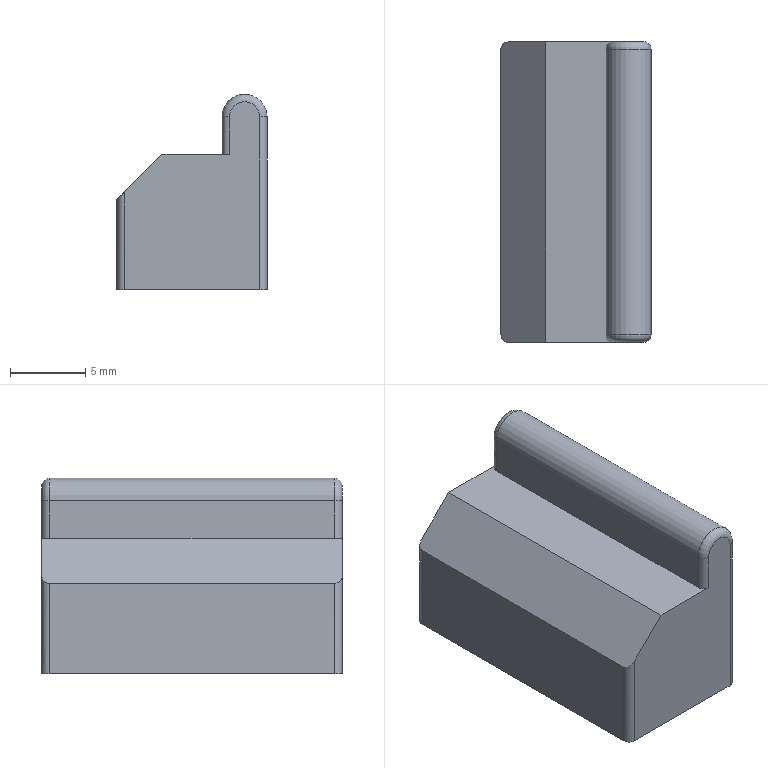NC program | Mastercam | posted with a generic post | part box 10 x 20 x 13 mm
Lines 868 to 2366 of 2366:
(4 BM/BNOS |TOOL - 14|DIA. OFF. - 14|LEN. - 14|TOOL DIA. - 4.)
N1800 T14 M6
N1802 G0 G54 G90 X-9.652 Y.005 C0. B0. S7000 M3
N1804 G43 H14 Z36.433
N1806 Z16.5
N1808 Z6.5
N1810 G1 Z-3.5 F600.
N1812 Y.021 Z-3.157 F3000.
N1814 Y.079 Z-2.784
N1816 Y.144 Z-2.521
N1818 Y.236 Z-2.248
N1820 Y.358 Z-1.968
N1822 Y.513 Z-1.685
N1824 Y.704 Z-1.403
N1826 Y.933 Z-1.128
N1828 Y1.131 Z-.93
N1830 Y1.351 Z-.743
N1832 Y1.593 Z-.571
N1834 Y1.855 Z-.416
N1836 Y2.136 Z-.282
N1838 Y2.434 Z-.171
N1840 Y2.744 Z-.087
N1842 Y3.065 Z-.032
N1844 Y3.391 Z-.006
N1846 Y3.718 Z-.011
N1848 Y4.043 Z-.047
N1850 Y4.36 Z-.112
N1852 Y4.667 Z-.205
N1854 Y4.959 Z-.324
N1856 Y5.235 Z-.465
N1858 Y5.49 Z-.627
N1860 Y5.725 Z-.804
N1862 Y5.938 Z-.995
N1864 Y6.187 Z-1.264
N1866 Y6.396 Z-1.543
N1868 Y6.569 Z-1.827
N1870 Y6.707 Z-2.109
N1872 Y6.813 Z-2.386
N1874 Y6.892 Z-2.654
N1876 Y6.964 Z-3.036
N1878 Y6.994 Z-3.389
N1880 Y6.995 Z-3.5
N1882 X-9.654 Y6.996 Z-3.53
N1884 X-9.66 Z-3.557
N1886 X-9.67 Y6.995 Z-3.579
N1888 X-9.684 Y6.994 Z-3.597
N1890 X-9.702 Y6.993 Z-3.612
N1892 X-9.724 Y6.991 Z-3.622
N1894 X-9.75 Y6.988 Z-3.628
N1896 X-9.781 Y6.985 Z-3.63
N1898 X-9.811 Y6.982 Z-3.628
N1900 X-9.837 Y6.979 Z-3.622
N1902 X-9.859 Y6.976 Z-3.611
N1904 X-9.877 Y6.974 Z-3.597
N1906 X-9.892 Y6.971 Z-3.579
N1908 X-9.902 Y6.97 Z-3.557
N1910 X-9.908 Y6.968 Z-3.53
N1912 X-9.91 Y6.966 Z-3.5
N1914 Y6.949 Z-3.16
N1916 Y6.893 Z-2.79
N1918 Y6.828 Z-2.529
N1920 Y6.736 Z-2.259
N1922 Y6.616 Z-1.981
N1924 Y6.462 Z-1.7
N1926 Y6.273 Z-1.42
N1928 Y6.046 Z-1.148
N1930 Y5.779 Z-.889
N1932 Y5.554 Z-.708
N1934 Y5.307 Z-.542
N1936 Y5.04 Z-.395
N1938 Y4.756 Z-.269
N1940 Y4.456 Z-.168
N1942 Y4.144 Z-.094
N1944 Y3.824 Z-.049
N1946 Y3.5 Z-.034
N1948 Y3.176 Z-.049
N1950 Y2.856 Z-.094
N1952 Y2.544 Z-.168
N1954 Y2.244 Z-.269
N1956 Y1.96 Z-.395
N1958 Y1.693 Z-.542
N1960 Y1.446 Z-.708
N1962 Y1.221 Z-.889
N1964 Y.954 Z-1.148
N1966 Y.727 Z-1.42
N1968 Y.538 Z-1.7
N1970 Y.384 Z-1.981
N1972 Y.264 Z-2.259
N1974 Y.172 Z-2.529
N1976 Y.107 Z-2.79
N1978 Y.051 Z-3.16
N1980 Y.034 Z-3.5
N1982 X-9.912 Y.033 Z-3.531
N1984 X-9.918 Z-3.559
N1986 X-9.928 Y.034 Z-3.582
N1988 X-9.942 Y.036 Z-3.601
N1990 X-9.961 Y.039 Z-3.615
N1992 X-9.983 Y.044 Z-3.626
N1994 X-10.01 Y.05 Z-3.632
N1996 X-10.041 Y.056 Z-3.634
N1998 X-10.072 Y.063 Z-3.632
N2000 X-10.098 Y.069 Z-3.626
N2002 X-10.121 Y.075 Z-3.615
N2004 X-10.139 Y.08 Z-3.601
N2006 X-10.153 Y.084 Z-3.582
N2008 X-10.164 Y.087 Z-3.559
N2010 X-10.17 Y.09 Z-3.531
N2012 X-10.172 Y.092 Z-3.5
N2014 Y.108 Z-3.166
N2016 Y.164 Z-2.802
N2018 Y.228 Z-2.546
N2020 Y.318 Z-2.28
N2022 Y.437 Z-2.007
N2024 Y.588 Z-1.73
N2026 Y.774 Z-1.455
N2028 Y.997 Z-1.187
N2030 Y1.259 Z-.932
N2032 Y1.481 Z-.755
N2034 Y1.724 Z-.592
N2036 Y1.986 Z-.447
N2038 Y2.265 Z-.324
N2040 Y2.56 Z-.224
N2042 Y2.867 Z-.151
N2044 Y3.181 Z-.107
N2046 Y3.5 Z-.092
N2048 Y3.819 Z-.107
N2050 Y4.133 Z-.151
N2052 Y4.44 Z-.224
N2054 Y4.735 Z-.324
N2056 Y5.014 Z-.447
N2058 Y5.276 Z-.592
N2060 Y5.519 Z-.755
N2062 Y5.741 Z-.932
N2064 Y6.003 Z-1.187
N2066 Y6.226 Z-1.455
N2068 Y6.412 Z-1.73
N2070 Y6.563 Z-2.007
N2072 Y6.682 Z-2.28
N2074 Y6.772 Z-2.546
N2076 Y6.836 Z-2.802
N2078 Y6.892 Z-3.166
N2080 Y6.908 Z-3.5
N2082 X-10.174 Y6.909 Z-3.532
N2084 X-10.18 Y6.908 Z-3.56
N2086 X-10.19 Y6.906 Z-3.584
N2088 X-10.205 Y6.902 Z-3.604
N2090 X-10.223 Y6.897 Z-3.619
N2092 X-10.245 Y6.889 Z-3.629
N2094 X-10.272 Y6.881 Z-3.636
N2096 X-10.303 Y6.87 Z-3.638
N2098 X-10.333 Y6.86 Z-3.636
N2100 X-10.36 Y6.851 Z-3.629
N2102 X-10.382 Y6.842 Z-3.619
N2104 X-10.401 Y6.835 Z-3.604
N2106 X-10.415 Y6.83 Z-3.584
N2108 X-10.425 Y6.825 Z-3.56
N2110 X-10.432 Y6.821 Z-3.532
N2112 X-10.434 Y6.819 Z-3.5
N2114 Y6.803 Z-3.174
N2116 Y6.749 Z-2.821
N2118 Y6.686 Z-2.571
N2120 Y6.599 Z-2.311
N2122 Y6.483 Z-2.046
N2124 Y6.337 Z-1.776
N2126 Y6.155 Z-1.509
N2128 Y5.938 Z-1.247
N2130 Y5.682 Z-.999
N2132 Y5.541 Z-.882
N2134 Y5.311 Z-.719
N2136 Y5.062 Z-.571
N2138 Y4.795 Z-.444
N2140 Y4.512 Z-.339
N2142 Y4.217 Z-.259
N2144 Y3.913 Z-.207
N2146 Y3.604 Z-.182
N2148 Y3.293 Z-.187
N2150 Y2.985 Z-.221
N2152 Y2.683 Z-.283
N2154 Y2.392 Z-.371
N2156 Y2.114 Z-.484
N2158 Y1.853 Z-.618
N2160 Y1.61 Z-.771
N2162 Y1.459 Z-.882
N2164 Y1.185 Z-1.121
N2166 Y.949 Z-1.377
N2168 Y.75 Z-1.642
N2170 Y.586 Z-1.911
N2172 Y.455 Z-2.179
N2174 Y.354 Z-2.442
N2176 Y.28 Z-2.697
N2178 Y.21 Z-3.059
N2180 Y.183 Z-3.395
N2182 Y.181 Z-3.5
N2184 X-10.436 Z-3.533
N2186 X-10.442 Y.183 Z-3.562
N2188 X-10.452 Y.187 Z-3.586
N2190 X-10.466 Y.193 Z-3.606
N2192 X-10.484 Y.201 Z-3.621
N2194 X-10.505 Y.211 Z-3.632
N2196 X-10.531 Y.222 Z-3.639
N2198 X-10.561 Y.236 Z-3.641
N2200 X-10.591 Y.25 Z-3.639
N2202 X-10.617 Y.263 Z-3.632
N2204 X-10.639 Y.273 Z-3.621
N2206 X-10.657 Y.282 Z-3.606
N2208 X-10.671 Y.289 Z-3.586
N2210 X-10.681 Y.295 Z-3.562
N2212 X-10.687 Y.299 Z-3.533
N2214 X-10.689 Y.301 Z-3.5
N2216 X-10.69 Y.317 Z-3.186
N2218 Y.369 Z-2.845
N2220 Y.429 Z-2.604
N2222 Y.513 Z-2.355
N2224 Y.625 Z-2.098
N2226 X-10.689 Y.766 Z-1.839
N2228 X-10.69 Y.941 Z-1.581
N2230 Y1.151 Z-1.329
N2232 Y1.397 Z-1.09
N2234 Y1.679 Z-.87
N2236 X-10.689 Y1.833 Z-.77
N2238 Y1.995 Z-.677
N2240 X-10.69 Y2.252 Z-.555
N2242 Y2.524 Z-.454
N2244 Y2.809 Z-.377
N2246 Y3.102 Z-.326
N2248 X-10.689 Y3.4 Z-.303
N2250 X-10.69 Y3.7 Z-.307
N2252 Y3.997 Z-.34
N2254 Y4.287 Z-.4
N2256 Y4.568 Z-.485
N2258 Y4.836 Z-.593
N2260 X-10.689 Y5.005 Z-.677
N2262 Y5.167 Z-.77
N2264 X-10.69 Y5.321 Z-.87
N2266 Y5.603 Z-1.09
N2268 Y5.849 Z-1.329
N2270 Y6.059 Z-1.581
N2272 X-10.689 Y6.234 Z-1.839
N2274 X-10.69 Y6.375 Z-2.098
N2276 Y6.487 Z-2.355
N2278 Y6.571 Z-2.604
N2280 Y6.653 Z-2.962
N2282 Y6.692 Z-3.294
N2284 X-10.689 Y6.699 Z-3.5
N2286 X-10.691 Z-3.534
N2288 X-10.697 Y6.696 Z-3.563
N2290 X-10.707 Y6.692 Z-3.588
N2292 X-10.72 Y6.684 Z-3.608
N2294 X-10.737 Y6.674 Z-3.623
N2296 X-10.758 Y6.662 Z-3.635
N2298 X-10.783 Y6.647 Z-3.641
N2300 X-10.812 Y6.629 Z-3.644
N2302 X-10.84 Y6.612 Z-3.641
N2304 X-10.865 Y6.596 Z-3.635
N2306 X-10.886 Y6.583 Z-3.623
N2308 X-10.903 Y6.571 Z-3.608
N2310 X-10.917 Y6.562 Z-3.587
N2312 X-10.926 Y6.555 Z-3.563
N2314 X-10.932 Y6.551 Z-3.534
N2316 X-10.934 Y6.548 Z-3.5
N2318 Y6.533 Z-3.201
N2320 Y6.483 Z-2.876
N2322 Y6.389 Z-2.529
N2324 Y6.296 Z-2.287
N2326 Y6.176 Z-2.041
N2328 Y6.025 Z-1.794
N2330 Y5.842 Z-1.55
N2332 X-10.935 Y5.625 Z-1.316
N2334 X-10.934 Y5.374 Z-1.097
N2336 Y5.089 Z-.899
N2338 Y4.934 Z-.811
N2340 Y4.772 Z-.731
N2342 Y4.604 Z-.659
N2344 Y4.43 Z-.598
N2346 X-10.935 Y4.25 Z-.546
N2348 X-10.934 Y4.066 Z-.506
N2350 Y3.879 Z-.476
N2352 Y3.69 Z-.458
N2354 Y3.5 Z-.452
N2356 Y3.31 Z-.458
N2358 Y3.121 Z-.476
N2360 Y2.934 Z-.506
N2362 X-10.935 Y2.75 Z-.546
N2364 X-10.934 Y2.57 Z-.598
N2366 Y2.396 Z-.659
N2368 Y2.228 Z-.731
N2370 Y2.066 Z-.811
N2372 Y1.911 Z-.899
N2374 Y1.626 Z-1.097
N2376 X-10.935 Y1.375 Z-1.316
N2378 X-10.934 Y1.158 Z-1.55
N2380 Y.975 Z-1.794
N2382 Y.824 Z-2.041
N2384 Y.704 Z-2.287
N2386 Y.611 Z-2.529
N2388 Y.517 Z-2.876
N2390 Y.467 Z-3.201
N2392 Y.452 Z-3.5
N2394 X-10.936 Z-3.534
N2396 X-10.941 Y.455 Z-3.563
N2398 X-10.95 Y.461 Z-3.588
N2400 X-10.962 Y.47 Z-3.609
N2402 X-10.978 Y.482 Z-3.625
N2404 X-10.998 Y.497 Z-3.636
N2406 X-11.021 Y.515 Z-3.643
N2408 X-11.048 Y.536 Z-3.645
N2410 X-11.074 Y.557 Z-3.643
N2412 X-11.098 Y.576 Z-3.636
N2414 X-11.117 Y.592 Z-3.625
N2416 X-11.133 Y.606 Z-3.609
N2418 X-11.146 Y.616 Z-3.588
N2420 X-11.155 Y.624 Z-3.563
N2422 X-11.16 Y.63 Z-3.534
N2424 X-11.162 Y.632 Z-3.5
N2426 Y.638 Z-3.315
N2428 Y.674 Z-3.017
N2430 Y.747 Z-2.697
N2432 Y.823 Z-2.473
N2434 Y.922 Z-2.243
N2436 Y1.049 Z-2.011
N2438 Y1.206 Z-1.779
N2440 Y1.394 Z-1.554
N2442 Y1.615 Z-1.34
N2444 Y1.867 Z-1.143
N2446 Y2.15 Z-.97
N2448 Y2.303 Z-.894
N2450 Y2.461 Z-.827
N2452 Y2.625 Z-.769
N2454 Y2.794 Z-.721
N2456 Y2.967 Z-.683
N2458 Y3.143 Z-.655
N2460 Y3.321 Z-.638
N2462 Y3.5 Z-.632
N2464 Y3.679 Z-.638
N2466 Y3.857 Z-.655
N2468 Y4.033 Z-.683
N2470 Y4.206 Z-.721
N2472 Y4.375 Z-.769
N2474 Y4.539 Z-.827
N2476 Y4.697 Z-.894
N2478 Y4.85 Z-.97
N2480 Y5.133 Z-1.143
N2482 Y5.385 Z-1.34
N2484 Y5.606 Z-1.554
N2486 Y5.794 Z-1.779
N2488 Y5.951 Z-2.011
N2490 Y6.078 Z-2.243
N2492 Y6.177 Z-2.473
N2494 Y6.282 Z-2.806
N2496 Y6.342 Z-3.119
N2498 Y6.362 Z-3.315
N2500 Y6.368 Z-3.5
N2502 X-11.163 Y6.367 Z-3.534
N2504 X-11.168 Y6.363 Z-3.564
N2506 X-11.176 Y6.356 Z-3.589
N2508 X-11.187 Y6.346 Z-3.609
N2510 X-11.202 Y6.332 Z-3.625
N2512 X-11.22 Y6.314 Z-3.636
N2514 X-11.241 Y6.294 Z-3.643
N2516 X-11.265 Y6.27 Z-3.646
N2518 X-11.289 Y6.245 Z-3.643
N2520 X-11.31 Y6.224 Z-3.636
N2522 X-11.327 Y6.206 Z-3.625
N2524 X-11.342 Y6.191 Z-3.609
N2526 X-11.353 Y6.179 Z-3.589
N2528 X-11.361 Y6.17 Z-3.564
N2530 X-11.366 Y6.164 Z-3.534
N2532 X-11.368 Y6.162 Z-3.5
N2534 Y6.156 Z-3.328
N2536 Y6.138 Z-3.147
N2538 Y6.105 Z-2.955
N2540 Y6.022 Z-2.652
N2542 Y5.892 Z-2.334
N2544 Y5.775 Z-2.118
N2546 Y5.629 Z-1.903
N2548 Y5.454 Z-1.694
N2550 Y5.25 Z-1.495
N2552 Y5.015 Z-1.312
N2554 Y4.753 Z-1.151
N2556 Y4.464 Z-1.019
N2558 Y4.155 Z-.921
N2560 Y3.995 Z-.885
N2562 Y3.831 Z-.859
N2564 Y3.666 Z-.844
N2566 Y3.5 Z-.838
N2568 Y3.334 Z-.844
N2570 Y3.169 Z-.859
N2572 Y3.005 Z-.885
N2574 Y2.688 Z-.966
N2576 Y2.389 Z-1.082
N2578 Y2.113 Z-1.228
N2580 Y1.864 Z-1.401
N2582 Y1.644 Z-1.593
N2584 Y1.454 Z-1.798
N2586 Y1.294 Z-2.01
N2588 Y1.163 Z-2.226
N2590 Y1.058 Z-2.441
N2592 Y.945 Z-2.755
N2594 Y.895 Z-2.955
N2596 Y.862 Z-3.147
N2598 Y.844 Z-3.328
N2600 Y.838 Z-3.5
N2602 X-11.369 Y.839 Z-3.534
N2604 X-11.373 Y.843 Z-3.563
N2606 X-11.38 Y.851 Z-3.588
N2608 X-11.39 Y.863 Z-3.609
N2610 X-11.403 Y.879 Z-3.625
N2612 X-11.418 Y.898 Z-3.636
N2614 X-11.437 Y.921 Z-3.643
N2616 X-11.458 Y.947 Z-3.645
N2618 X-11.479 Y.974 Z-3.643
N2620 X-11.497 Y.997 Z-3.636
N2622 X-11.513 Y1.017 Z-3.625
N2624 X-11.525 Y1.034 Z-3.609
N2626 X-11.535 Y1.047 Z-3.588
N2628 X-11.542 Y1.057 Z-3.563
N2630 X-11.546 Y1.063 Z-3.534
N2632 X-11.548 Y1.066 Z-3.5
N2634 Y1.071 Z-3.343
N2636 Y1.088 Z-3.177
N2638 Y1.118 Z-3.002
N2640 Y1.164 Z-2.819
N2642 Y1.228 Z-2.629
N2644 Y1.363 Z-2.335
N2646 Y1.483 Z-2.138
N2648 Y1.63 Z-1.943
N2650 Y1.803 Z-1.756
N2652 Y2.004 Z-1.581
N2654 Y2.231 Z-1.423
N2656 Y2.484 Z-1.289
N2658 Y2.758 Z-1.183
N2660 Y3.048 Z-1.109
N2662 Y3.348 Z-1.071
N2664 Y3.652
N2666 Y3.952 Z-1.109
N2668 Y4.242 Z-1.183
N2670 Y4.516 Z-1.289
N2672 Y4.769 Z-1.423
N2674 Y4.996 Z-1.581
N2676 Y5.197 Z-1.756
N2678 Y5.37 Z-1.943
N2680 Y5.517 Z-2.138
N2682 Y5.637 Z-2.335
N2684 Y5.772 Z-2.629
N2686 Y5.836 Z-2.819
N2688 Y5.882 Z-3.002
N2690 Y5.912 Z-3.177
N2692 Y5.929 Z-3.343
N2694 Y5.934 Z-3.5
N2696 X-11.549 Y5.933 Z-3.534
N2698 X-11.553 Y5.929 Z-3.563
N2700 X-11.558 Y5.92 Z-3.587
N2702 X-11.567 Y5.908 Z-3.608
N2704 X-11.577 Y5.892 Z-3.623
N2706 X-11.59 Y5.872 Z-3.635
N2708 X-11.606 Y5.847 Z-3.641
N2710 X-11.623 Y5.819 Z-3.644
N2712 X-11.641 Y5.79 Z-3.641
N2714 X-11.656 Y5.765 Z-3.635
N2716 X-11.669 Y5.744 Z-3.623
N2718 X-11.68 Y5.726 Z-3.608
N2720 X-11.688 Y5.712 Z-3.587
N2722 X-11.694 Y5.701 Z-3.563
N2724 X-11.698 Y5.694 Z-3.534
N2726 X-11.699 Y5.689 Z-3.5
N2728 Y5.67 Z-3.209
N2730 Y5.642 Z-3.052
N2732 Y5.601 Z-2.887
N2734 Y5.544 Z-2.716
N2736 Y5.468 Z-2.541
N2738 Y5.371 Z-2.363
N2740 Y5.251 Z-2.187
N2742 Y5.107 Z-2.015
N2744 Y4.939 Z-1.851
N2746 Y4.747 Z-1.7
N2748 Y4.53 Z-1.568
N2750 Y4.293 Z-1.46
N2752 Y4.039 Z-1.379
N2754 Y3.773 Z-1.328
N2756 Y3.5 Z-1.311
N2758 Y3.227 Z-1.328
N2760 Y2.961 Z-1.379
N2762 Y2.707 Z-1.46
N2764 Y2.47 Z-1.568
N2766 Y2.253 Z-1.7
N2768 Y2.154 Z-1.774
N2770 Y1.974 Z-1.931
N2772 Y1.818 Z-2.1
N2774 Y1.686 Z-2.274
N2776 Y1.532 Z-2.541
N2778 Y1.456 Z-2.716
N2780 Y1.399 Z-2.887
N2782 Y1.358 Z-3.052
N2784 Y1.33 Z-3.209
N2786 Y1.311 Z-3.5
N2788 X-11.7 Y1.31 Z-3.533
N2790 X-11.703 Y1.314 Z-3.562
N2792 X-11.707 Y1.323 Z-3.586
N2794 X-11.714 Y1.335 Z-3.606
N2796 X-11.722 Y1.352 Z-3.621
N2798 X-11.733 Y1.373 Z-3.632
N2800 X-11.745 Y1.399 Z-3.639
N2802 X-11.759 Y1.429 Z-3.641
N2804 X-11.773 Y1.459 Z-3.639
N2806 X-11.785 Y1.485 Z-3.632
N2808 X-11.796 Y1.508 Z-3.621
N2810 X-11.804 Y1.527 Z-3.606
N2812 X-11.811 Y1.543 Z-3.586
N2814 X-11.815 Y1.554 Z-3.562
N2816 X-11.818 Y1.562 Z-3.533
N2818 X-11.819 Y1.566 Z-3.5
N2820 Y1.584 Z-3.243
N2822 Y1.608 Z-3.104
N2824 X-11.82 Y1.645 Z-2.959
N2826 X-11.819 Y1.695 Z-2.808
N2828 Y1.802 Z-2.574
N2830 Y1.898 Z-2.418
N2832 Y2.014 Z-2.264
N2834 X-11.82 Y2.152 Z-2.115
N2836 X-11.819 Y2.311 Z-1.976
N2838 Y2.492 Z-1.85
N2840 Y2.693 Z-1.743
N2842 Y2.91 Z-1.659
N2844 Y3.141 Z-1.601
N2846 Y3.379 Z-1.57
N2848 Y3.621
N2850 Y3.859 Z-1.601
N2852 Y4.09 Z-1.659
N2854 Y4.307 Z-1.743
N2856 Y4.508 Z-1.85
N2858 Y4.689 Z-1.976
N2860 X-11.82 Y4.848 Z-2.115
N2862 X-11.819 Y4.986 Z-2.264
N2864 Y5.102 Z-2.418
N2866 Y5.198 Z-2.574
N2868 Y5.305 Z-2.808
N2870 X-11.82 Y5.355 Z-2.959
N2872 X-11.819 Y5.392 Z-3.104
N2874 Y5.416 Z-3.243
N2876 Y5.434 Z-3.5
N2878 X-11.82 Z-3.532
N2880 X-11.822 Y5.43 Z-3.56
N2882 X-11.825 Y5.421 Z-3.584
N2884 X-11.83 Y5.408 Z-3.603
N2886 X-11.836 Y5.391 Z-3.618
N2888 X-11.844 Y5.369 Z-3.629
N2890 X-11.853 Y5.343 Z-3.636
N2892 X-11.863 Y5.312 Z-3.638
N2894 X-11.874 Y5.281 Z-3.636
N2896 X-11.883 Y5.254 Z-3.629
N2898 X-11.891 Y5.231 Z-3.618
N2900 X-11.897 Y5.212 Z-3.603
N2902 X-11.902 Y5.196 Z-3.584
N2904 X-11.905 Y5.184 Z-3.56
N2906 X-11.907 Y5.176 Z-3.532
N2908 X-11.908 Y5.172 Z-3.5
N2910 Y5.157 Z-3.278
N2912 Y5.104 Z-3.032
N2914 Y5.06 Z-2.902
N2916 Y4.968 Z-2.7
N2918 Y4.837 Z-2.497
N2920 Y4.665 Z-2.302
N2922 Y4.528 Z-2.182
N2924 Y4.371 Z-2.073
N2926 Y4.198 Z-1.981
N2928 Y4.01 Z-1.909
N2930 Y3.811 Z-1.858
N2932 Y3.604 Z-1.832
N2934 Y3.396
N2936 Y3.189 Z-1.858
N2938 Y2.99 Z-1.909
N2940 Y2.802 Z-1.981
N2942 Y2.629 Z-2.073
N2944 Y2.472 Z-2.182
N2946 Y2.273 Z-2.366
N2948 Y2.115 Z-2.564
N2950 Y1.997 Z-2.767
N2952 Y1.94 Z-2.902
N2954 Y1.896 Z-3.032
N2956 Y1.843 Z-3.278
N2958 Y1.828 Z-3.5
N2960 Z-3.531
N2962 X-11.91 Y1.832 Z-3.559
N2964 X-11.912 Y1.841 Z-3.582
N2966 X-11.915 Y1.854 Z-3.6
N2968 X-11.919 Y1.871 Z-3.615
N2970 X-11.924 Y1.893 Z-3.626
N2972 X-11.93 Y1.919 Z-3.632
N2974 X-11.937 Y1.95 Z-3.634
N2976 X-11.944 Y1.981 Z-3.632
N2978 X-11.95 Y2.008 Z-3.626
N2980 X-11.955 Y2.031 Z-3.615
N2982 X-11.959 Y2.051 Z-3.6
N2984 X-11.962 Y2.066 Z-3.582
N2986 X-11.964 Y2.078 Z-3.559
N2988 X-11.966 Y2.086 Z-3.531
N2990 Y2.09 Z-3.5
N2992 Y2.103 Z-3.313
N2994 Y2.148 Z-3.106
N2996 Y2.233 Z-2.882
N2998 Y2.295 Z-2.768
N3000 Y2.417 Z-2.599
N3002 Y2.574 Z-2.439
N3004 Y2.765 Z-2.297
N3006 Y2.912 Z-2.219
N3008 Y3.07 Z-2.158
N3010 Y3.238 Z-2.116
N3012 Y3.412 Z-2.093
N3014 Y3.588
N3016 Y3.762 Z-2.116
N3018 Y3.93 Z-2.158
N3020 Y4.088 Z-2.219
N3022 Y4.235 Z-2.297
N3024 Y4.426 Z-2.439
N3026 Y4.583 Z-2.599
N3028 Y4.705 Z-2.768
N3030 Y4.767 Z-2.882
N3032 Y4.852 Z-3.106
N3034 Y4.897 Z-3.313
N3036 Y4.91 Z-3.5
N3038 Z-3.53
N3040 X-11.967 Y4.906 Z-3.557
N3042 X-11.968 Y4.897 Z-3.579
N3044 X-11.97 Y4.884 Z-3.597
N3046 X-11.972 Y4.867 Z-3.611
N3048 X-11.974 Y4.846 Z-3.621
N3050 X-11.977 Y4.82 Z-3.627
N3052 X-11.981 Y4.79 Z-3.629
N3054 X-11.984 Y4.759 Z-3.627
N3056 X-11.987 Y4.733 Z-3.621
N3058 X-11.99 Y4.71 Z-3.611
N3060 X-11.992 Y4.691 Z-3.597
N3062 X-11.993 Y4.675 Z-3.579
N3064 X-11.994 Y4.664 Z-3.557
N3066 X-11.995 Y4.656 Z-3.53
N3068 Y4.652 Z-3.5
N3070 Y4.641 Z-3.347
N3072 Y4.605 Z-3.178
N3074 Y4.535 Z-2.995
N3076 Y4.484 Z-2.902
N3078 Y4.385 Z-2.764
N3080 Y4.257 Z-2.633
N3082 Y4.1 Z-2.517
N3084 Y3.917 Z-2.427
N3086 Y3.714 Z-2.369
N3088 Y3.5 Z-2.348
N3090 Y3.286 Z-2.369
N3092 Y3.083 Z-2.427
N3094 Y2.9 Z-2.517
N3096 Y2.743 Z-2.633
N3098 Y2.615 Z-2.764
N3100 Y2.516 Z-2.902
N3102 Y2.425 Z-3.088
N3104 Y2.374 Z-3.264
N3106 Y2.351 Z-3.426
N3108 Y2.348 Z-3.5
N3110 G0 Z6.5
N3112 Z16.5
N3114 Z36.433
N3116 X9.652 Y6.995
N3118 Z16.5
N3120 Z6.5
N3122 G1 Z-3.5 F600.
N3124 Y6.979 Z-3.157 F3000.
N3126 Y6.921 Z-2.784
N3128 Y6.856 Z-2.521
N3130 Y6.764 Z-2.248
N3132 Y6.642 Z-1.968
N3134 Y6.487 Z-1.685
N3136 Y6.296 Z-1.403
N3138 Y6.067 Z-1.128
N3140 Y5.869 Z-.93
N3142 Y5.649 Z-.743
N3144 Y5.407 Z-.571
N3146 Y5.145 Z-.416
N3148 Y4.864 Z-.282
N3150 Y4.566 Z-.171
N3152 Y4.256 Z-.087
N3154 Y3.935 Z-.032
N3156 Y3.609 Z-.006
N3158 Y3.282 Z-.011
N3160 Y2.957 Z-.047
N3162 Y2.64 Z-.112
N3164 Y2.333 Z-.205
N3166 Y2.041 Z-.324
N3168 Y1.765 Z-.465
N3170 Y1.51 Z-.627
N3172 Y1.275 Z-.804
N3174 Y1.062 Z-.995
N3176 Y.813 Z-1.264
N3178 Y.604 Z-1.543
N3180 Y.431 Z-1.827
N3182 Y.293 Z-2.109
N3184 Y.187 Z-2.386
N3186 Y.108 Z-2.654
N3188 Y.036 Z-3.036
N3190 Y.006 Z-3.389
N3192 Y.005 Z-3.5
N3194 X9.654 Y.004 Z-3.53
N3196 X9.66 Z-3.557
N3198 X9.67 Y.005 Z-3.579
N3200 X9.684 Y.006 Z-3.597
N3202 X9.702 Y.007 Z-3.612
N3204 X9.724 Y.009 Z-3.622
N3206 X9.75 Y.012 Z-3.628
N3208 X9.781 Y.015 Z-3.63
N3210 X9.811 Y.018 Z-3.628
N3212 X9.837 Y.021 Z-3.622
N3214 X9.859 Y.024 Z-3.611
N3216 X9.877 Y.026 Z-3.597
N3218 X9.892 Y.029 Z-3.579
N3220 X9.902 Y.03 Z-3.557
N3222 X9.908 Y.032 Z-3.53
N3224 X9.91 Y.034 Z-3.5
N3226 Y.051 Z-3.16
N3228 Y.107 Z-2.79
N3230 Y.172 Z-2.529
N3232 Y.264 Z-2.259
N3234 Y.384 Z-1.981
N3236 Y.538 Z-1.7
N3238 Y.727 Z-1.42
N3240 Y.954 Z-1.148
N3242 Y1.221 Z-.889
N3244 Y1.446 Z-.708
N3246 Y1.693 Z-.542
N3248 Y1.96 Z-.395
N3250 Y2.244 Z-.269
N3252 Y2.544 Z-.168
N3254 Y2.856 Z-.094
N3256 Y3.176 Z-.049
N3258 Y3.5 Z-.034
N3260 Y3.824 Z-.049
N3262 Y4.144 Z-.094
N3264 Y4.456 Z-.168
N3266 Y4.756 Z-.269
N3268 Y5.04 Z-.395
N3270 Y5.307 Z-.542
N3272 Y5.554 Z-.708
N3274 Y5.779 Z-.889
N3276 Y6.046 Z-1.148
N3278 Y6.273 Z-1.42
N3280 Y6.462 Z-1.7
N3282 Y6.616 Z-1.981
N3284 Y6.736 Z-2.259
N3286 Y6.828 Z-2.529
N3288 Y6.893 Z-2.79
N3290 Y6.949 Z-3.16
N3292 Y6.966 Z-3.5
N3294 X9.912 Y6.967 Z-3.531
N3296 X9.918 Z-3.559
N3298 X9.928 Y6.966 Z-3.582
N3300 X9.942 Y6.964 Z-3.601
N3302 X9.961 Y6.961 Z-3.615
N3304 X9.983 Y6.956 Z-3.626
N3306 X10.01 Y6.95 Z-3.632
N3308 X10.041 Y6.944 Z-3.634
N3310 X10.072 Y6.937 Z-3.632
N3312 X10.098 Y6.931 Z-3.626
N3314 X10.121 Y6.925 Z-3.615
N3316 X10.139 Y6.92 Z-3.601
N3318 X10.153 Y6.916 Z-3.582
N3320 X10.164 Y6.913 Z-3.559
N3322 X10.17 Y6.91 Z-3.531
N3324 X10.172 Y6.908 Z-3.5
N3326 Y6.892 Z-3.166
N3328 Y6.836 Z-2.802
N3330 Y6.772 Z-2.546
N3332 Y6.682 Z-2.28
N3334 Y6.563 Z-2.007
N3336 Y6.412 Z-1.73
N3338 Y6.226 Z-1.455
N3340 Y6.003 Z-1.187
N3342 Y5.741 Z-.932
N3344 Y5.519 Z-.755
N3346 Y5.276 Z-.592
N3348 Y5.014 Z-.447
N3350 Y4.735 Z-.324
N3352 Y4.44 Z-.224
N3354 Y4.133 Z-.151
N3356 Y3.819 Z-.107
N3358 Y3.5 Z-.092
N3360 Y3.181 Z-.107
N3362 Y2.867 Z-.151
N3364 Y2.56 Z-.224
N3366 Y2.265 Z-.324
N3368 Y1.986 Z-.447
N3370 Y1.724 Z-.592
N3372 Y1.481 Z-.755
N3374 Y1.259 Z-.932
N3376 Y.997 Z-1.187
N3378 Y.774 Z-1.455
N3380 Y.588 Z-1.73
N3382 Y.437 Z-2.007
N3384 Y.318 Z-2.28
N3386 Y.228 Z-2.546
N3388 Y.164 Z-2.802
N3390 Y.108 Z-3.166
N3392 Y.092 Z-3.5
N3394 X10.174 Y.091 Z-3.532
N3396 X10.18 Y.092 Z-3.56
N3398 X10.19 Y.094 Z-3.584
N3400 X10.205 Y.098 Z-3.604
N3402 X10.223 Y.103 Z-3.619
N3404 X10.245 Y.111 Z-3.629
N3406 X10.272 Y.119 Z-3.636
N3408 X10.303 Y.13 Z-3.638
N3410 X10.333 Y.14 Z-3.636
N3412 X10.36 Y.149 Z-3.629
N3414 X10.382 Y.158 Z-3.619
N3416 X10.401 Y.165 Z-3.604
N3418 X10.415 Y.17 Z-3.584
N3420 X10.425 Y.175 Z-3.56
N3422 X10.432 Y.179 Z-3.532
N3424 X10.434 Y.181 Z-3.5
N3426 Y.197 Z-3.174
N3428 Y.251 Z-2.821
N3430 Y.314 Z-2.571
N3432 Y.401 Z-2.311
N3434 Y.517 Z-2.046
N3436 Y.663 Z-1.776
N3438 Y.845 Z-1.509
N3440 Y1.062 Z-1.247
N3442 Y1.318 Z-.999
N3444 Y1.459 Z-.882
N3446 Y1.689 Z-.719
N3448 Y1.938 Z-.571
N3450 Y2.205 Z-.444
N3452 Y2.488 Z-.339
N3454 Y2.783 Z-.259
N3456 Y3.087 Z-.207
N3458 Y3.396 Z-.182
N3460 Y3.707 Z-.187
N3462 Y4.015 Z-.221
N3464 Y4.317 Z-.283
N3466 Y4.608 Z-.371
N3468 Y4.886 Z-.484
N3470 Y5.147 Z-.618
N3472 Y5.39 Z-.771
N3474 Y5.541 Z-.882
N3476 Y5.815 Z-1.121
N3478 Y6.051 Z-1.377
N3480 Y6.25 Z-1.642
N3482 Y6.414 Z-1.911
N3484 Y6.545 Z-2.179
N3486 Y6.646 Z-2.442
N3488 Y6.72 Z-2.697
N3490 Y6.79 Z-3.059
N3492 Y6.817 Z-3.395
N3494 Y6.819 Z-3.5
N3496 X10.436 Z-3.533
N3498 X10.442 Y6.817 Z-3.562
N3500 X10.452 Y6.813 Z-3.586
N3502 X10.466 Y6.807 Z-3.606
N3504 X10.484 Y6.799 Z-3.621
N3506 X10.505 Y6.789 Z-3.632
N3508 X10.531 Y6.778 Z-3.639
N3510 X10.561 Y6.764 Z-3.641
N3512 X10.591 Y6.75 Z-3.639
N3514 X10.617 Y6.737 Z-3.632
N3516 X10.639 Y6.727 Z-3.621
N3518 X10.657 Y6.718 Z-3.606
N3520 X10.671 Y6.711 Z-3.586
N3522 X10.681 Y6.705 Z-3.562
N3524 X10.687 Y6.701 Z-3.533
N3526 X10.689 Y6.699 Z-3.5
N3528 X10.69 Y6.683 Z-3.186
N3530 Y6.631 Z-2.845
N3532 Y6.571 Z-2.604
N3534 Y6.487 Z-2.355
N3536 Y6.375 Z-2.098
N3538 X10.689 Y6.234 Z-1.839
N3540 X10.69 Y6.059 Z-1.581
N3542 Y5.849 Z-1.329
N3544 Y5.603 Z-1.09
N3546 Y5.321 Z-.87
N3548 X10.689 Y5.167 Z-.77
N3550 Y5.005 Z-.677
N3552 X10.69 Y4.748 Z-.555
N3554 Y4.476 Z-.454
N3556 Y4.191 Z-.377
N3558 Y3.898 Z-.326
N3560 X10.689 Y3.6 Z-.303
N3562 X10.69 Y3.3 Z-.307
N3564 Y3.003 Z-.34
N3566 Y2.713 Z-.4
N3568 Y2.432 Z-.485
N3570 Y2.164 Z-.593
N3572 X10.689 Y1.995 Z-.677
N3574 Y1.833 Z-.77
N3576 X10.69 Y1.679 Z-.87
N3578 Y1.397 Z-1.09
N3580 Y1.151 Z-1.329
N3582 Y.941 Z-1.581
N3584 X10.689 Y.766 Z-1.839
N3586 X10.69 Y.625 Z-2.098
N3588 Y.513 Z-2.355
N3590 Y.429 Z-2.604
N3592 Y.347 Z-2.962
N3594 Y.308 Z-3.294
N3596 X10.689 Y.301 Z-3.5
N3598 X10.691 Z-3.534
N3600 X10.697 Y.304 Z-3.563
N3602 X10.707 Y.308 Z-3.588
N3604 X10.72 Y.316 Z-3.608
N3606 X10.737 Y.326 Z-3.623
N3608 X10.758 Y.338 Z-3.635
N3610 X10.783 Y.353 Z-3.641
N3612 X10.812 Y.371 Z-3.644
N3614 X10.84 Y.388 Z-3.641
N3616 X10.865 Y.404 Z-3.635
N3618 X10.886 Y.417 Z-3.623
N3620 X10.903 Y.429 Z-3.608
N3622 X10.917 Y.438 Z-3.587
N3624 X10.926 Y.445 Z-3.563
N3626 X10.932 Y.449 Z-3.534
N3628 X10.934 Y.452 Z-3.5
N3630 Y.467 Z-3.201
N3632 Y.517 Z-2.876
N3634 Y.611 Z-2.529
N3636 Y.704 Z-2.287
N3638 Y.824 Z-2.041
N3640 Y.975 Z-1.794
N3642 Y1.158 Z-1.55
N3644 X10.935 Y1.375 Z-1.316
N3646 X10.934 Y1.626 Z-1.097
N3648 Y1.911 Z-.899
N3650 Y2.066 Z-.811
N3652 Y2.228 Z-.731
N3654 Y2.396 Z-.659
N3656 Y2.57 Z-.598
N3658 X10.935 Y2.75 Z-.546
N3660 X10.934 Y2.934 Z-.506
N3662 Y3.121 Z-.476
N3664 Y3.31 Z-.458
N3666 Y3.5 Z-.452
N3668 Y3.69 Z-.458
N3670 Y3.879 Z-.476
N3672 Y4.066 Z-.506
N3674 X10.935 Y4.25 Z-.546
N3676 X10.934 Y4.43 Z-.598
N3678 Y4.604 Z-.659
N3680 Y4.772 Z-.731
N3682 Y4.934 Z-.811
N3684 Y5.089 Z-.899
N3686 Y5.374 Z-1.097
N3688 X10.935 Y5.625 Z-1.316
N3690 X10.934 Y5.842 Z-1.55
N3692 Y6.025 Z-1.794
N3694 Y6.176 Z-2.041
N3696 Y6.296 Z-2.287
N3698 Y6.389 Z-2.529
N3700 Y6.483 Z-2.876
N3702 Y6.533 Z-3.201
N3704 Y6.548 Z-3.5
N3706 X10.936 Z-3.534
N3708 X10.941 Y6.545 Z-3.563
N3710 X10.95 Y6.539 Z-3.588
N3712 X10.962 Y6.53 Z-3.609
N3714 X10.978 Y6.518 Z-3.625
N3716 X10.998 Y6.503 Z-3.636
N3718 X11.021 Y6.485 Z-3.643
N3720 X11.048 Y6.464 Z-3.645
N3722 X11.074 Y6.443 Z-3.643
N3724 X11.098 Y6.424 Z-3.636
N3726 X11.117 Y6.408 Z-3.625
N3728 X11.133 Y6.394 Z-3.609
N3730 X11.146 Y6.384 Z-3.588
N3732 X11.155 Y6.376 Z-3.563
N3734 X11.16 Y6.37 Z-3.534
N3736 X11.162 Y6.368 Z-3.5
N3738 Y6.362 Z-3.315
N3740 Y6.326 Z-3.017
N3742 Y6.253 Z-2.697
N3744 Y6.177 Z-2.473
N3746 Y6.078 Z-2.243
N3748 Y5.951 Z-2.011
N3750 Y5.794 Z-1.779
N3752 Y5.606 Z-1.554
N3754 Y5.385 Z-1.34
N3756 Y5.133 Z-1.143
N3758 Y4.85 Z-.97
N3760 Y4.697 Z-.894
N3762 Y4.539 Z-.827
N3764 Y4.375 Z-.769
N3766 Y4.206 Z-.721
N3768 Y4.033 Z-.683
N3770 Y3.857 Z-.655
N3772 Y3.679 Z-.638
N3774 Y3.5 Z-.632
N3776 Y3.321 Z-.638
N3778 Y3.143 Z-.655
N3780 Y2.967 Z-.683
N3782 Y2.794 Z-.721
N3784 Y2.625 Z-.769
N3786 Y2.461 Z-.827
N3788 Y2.303 Z-.894
N3790 Y2.15 Z-.97
N3792 Y1.867 Z-1.143
N3794 Y1.615 Z-1.34
N3796 Y1.394 Z-1.554
N3798 Y1.206 Z-1.779
N3800 Y1.049 Z-2.011
N3802 Y.922 Z-2.243
N3804 Y.823 Z-2.473
N3806 Y.718 Z-2.806
N3808 Y.658 Z-3.119
N3810 Y.638 Z-3.315
N3812 Y.632 Z-3.5
N3814 X11.163 Y.633 Z-3.534
N3816 X11.168 Y.637 Z-3.564
N3818 X11.176 Y.644 Z-3.589
N3820 X11.187 Y.654 Z-3.609
N3822 X11.202 Y.668 Z-3.625
N3824 X11.22 Y.686 Z-3.636
N3826 X11.241 Y.706 Z-3.643
N3828 X11.265 Y.73 Z-3.646
N3830 X11.289 Y.755 Z-3.643
N3832 X11.31 Y.776 Z-3.636
N3834 X11.327 Y.794 Z-3.625
N3836 X11.342 Y.809 Z-3.609
N3838 X11.353 Y.821 Z-3.589
N3840 X11.361 Y.83 Z-3.564
N3842 X11.366 Y.836 Z-3.534
N3844 X11.368 Y.838 Z-3.5
N3846 Y.844 Z-3.328
N3848 Y.862 Z-3.147
N3850 Y.895 Z-2.955
N3852 Y.978 Z-2.652
N3854 Y1.108 Z-2.334
N3856 Y1.225 Z-2.118
N3858 Y1.371 Z-1.903
N3860 Y1.546 Z-1.694
N3862 Y1.75 Z-1.495
N3864 Y1.985 Z-1.312
N3866 Y2.247 Z-1.151
N3868 Y2.536 Z-1.019
N3870 Y2.845 Z-.921
N3872 Y3.005 Z-.885
N3874 Y3.169 Z-.859
N3876 Y3.334 Z-.844
N3878 Y3.5 Z-.838
N3880 Y3.666 Z-.844
N3882 Y3.831 Z-.859
N3884 Y3.995 Z-.885
N3886 Y4.312 Z-.966
N3888 Y4.611 Z-1.082
N3890 Y4.887 Z-1.228
N3892 Y5.136 Z-1.401
N3894 Y5.356 Z-1.593
N3896 Y5.546 Z-1.798
N3898 Y5.706 Z-2.01
N3900 Y5.837 Z-2.226
N3902 Y5.942 Z-2.441
N3904 Y6.055 Z-2.755
N3906 Y6.105 Z-2.955
N3908 Y6.138 Z-3.147
N3910 Y6.156 Z-3.328
N3912 Y6.162 Z-3.5
N3914 X11.369 Y6.161 Z-3.534
N3916 X11.373 Y6.157 Z-3.563
N3918 X11.38 Y6.149 Z-3.588
N3920 X11.39 Y6.137 Z-3.609
N3922 X11.403 Y6.121 Z-3.625
N3924 X11.418 Y6.102 Z-3.636
N3926 X11.437 Y6.079 Z-3.643
N3928 X11.458 Y6.053 Z-3.645
N3930 X11.479 Y6.026 Z-3.643
N3932 X11.497 Y6.003 Z-3.636
N3934 X11.513 Y5.983 Z-3.625
N3936 X11.525 Y5.966 Z-3.609
N3938 X11.535 Y5.953 Z-3.588
N3940 X11.542 Y5.943 Z-3.563
N3942 X11.546 Y5.937 Z-3.534
N3944 X11.548 Y5.934 Z-3.5
N3946 Y5.929 Z-3.343
N3948 Y5.912 Z-3.177
N3950 Y5.882 Z-3.002
N3952 Y5.836 Z-2.819
N3954 Y5.772 Z-2.629
N3956 Y5.637 Z-2.335
N3958 Y5.517 Z-2.138
N3960 Y5.37 Z-1.943
N3962 Y5.197 Z-1.756
N3964 Y4.996 Z-1.581
N3966 Y4.769 Z-1.423
N3968 Y4.516 Z-1.289
N3970 Y4.242 Z-1.183
N3972 Y3.952 Z-1.109
N3974 Y3.652 Z-1.071
N3976 Y3.348
N3978 Y3.048 Z-1.109
N3980 Y2.758 Z-1.183
N3982 Y2.484 Z-1.289
N3984 Y2.231 Z-1.423
N3986 Y2.004 Z-1.581
N3988 Y1.803 Z-1.756
N3990 Y1.63 Z-1.943
N3992 Y1.483 Z-2.138
N3994 Y1.363 Z-2.335
N3996 Y1.228 Z-2.629
N3998 Y1.164 Z-2.819
N4000 Y1.118 Z-3.002
N4002 Y1.088 Z-3.177
N4004 Y1.071 Z-3.343
N4006 Y1.066 Z-3.5
N4008 X11.549 Y1.067 Z-3.534
N4010 X11.553 Y1.071 Z-3.563
N4012 X11.558 Y1.08 Z-3.587
N4014 X11.567 Y1.092 Z-3.608
N4016 X11.577 Y1.108 Z-3.623
N4018 X11.59 Y1.128 Z-3.635
N4020 X11.606 Y1.153 Z-3.641
N4022 X11.623 Y1.181 Z-3.644
N4024 X11.641 Y1.21 Z-3.641
N4026 X11.656 Y1.235 Z-3.635
N4028 X11.669 Y1.256 Z-3.623
N4030 X11.68 Y1.274 Z-3.608
N4032 X11.688 Y1.288 Z-3.587
N4034 X11.694 Y1.299 Z-3.563
N4036 X11.698 Y1.306 Z-3.534
N4038 X11.699 Y1.311 Z-3.5
N4040 Y1.33 Z-3.209
N4042 Y1.358 Z-3.052
N4044 Y1.399 Z-2.887
N4046 Y1.456 Z-2.716
N4048 Y1.578 Z-2.452
N4050 Y1.686 Z-2.274
N4052 Y1.818 Z-2.1
N4054 Y1.974 Z-1.931
N4056 Y2.154 Z-1.774
N4058 Y2.359 Z-1.632
N4060 Y2.586 Z-1.511
N4062 Y2.832 Z-1.416
N4064 Y3.093 Z-1.349
N4066 Y3.363 Z-1.315
N4068 Y3.637
N4070 Y3.907 Z-1.349
N4072 Y4.168 Z-1.416
N4074 Y4.414 Z-1.511
N4076 Y4.641 Z-1.632
N4078 Y4.846 Z-1.774
N4080 Y4.939 Z-1.851
N4082 Y5.107 Z-2.015
N4084 Y5.251 Z-2.187
N4086 Y5.371 Z-2.363
N4088 Y5.468 Z-2.541
N4090 Y5.544 Z-2.716
N4092 Y5.601 Z-2.887
N4094 Y5.642 Z-3.052
N4096 Y5.67 Z-3.209
N4098 Y5.689 Z-3.5
N4100 X11.7 Y5.69 Z-3.533
N4102 X11.703 Y5.686 Z-3.562
N4104 X11.707 Y5.677 Z-3.586
N4106 X11.714 Y5.665 Z-3.606
N4108 X11.722 Y5.648 Z-3.621
N4110 X11.733 Y5.627 Z-3.632
N4112 X11.745 Y5.601 Z-3.639
N4114 X11.759 Y5.571 Z-3.641
N4116 X11.773 Y5.541 Z-3.639
N4118 X11.785 Y5.515 Z-3.632
N4120 X11.796 Y5.492 Z-3.621
N4122 X11.804 Y5.473 Z-3.606
N4124 X11.811 Y5.457 Z-3.586
N4126 X11.815 Y5.446 Z-3.562
N4128 X11.818 Y5.438 Z-3.533
N4130 X11.819 Y5.434 Z-3.5
N4132 Y5.416 Z-3.243
N4134 Y5.392 Z-3.104
N4136 X11.82 Y5.355 Z-2.959
N4138 X11.819 Y5.305 Z-2.808
N4140 Y5.198 Z-2.574
N4142 Y5.102 Z-2.418
N4144 Y4.986 Z-2.264
N4146 X11.82 Y4.848 Z-2.115
N4148 X11.819 Y4.689 Z-1.976
N4150 Y4.508 Z-1.85
N4152 Y4.307 Z-1.743
N4154 Y4.09 Z-1.659
N4156 Y3.859 Z-1.601
N4158 Y3.621 Z-1.57
N4160 Y3.379
N4162 Y3.141 Z-1.601
N4164 Y2.91 Z-1.659
N4166 Y2.693 Z-1.743
N4168 Y2.492 Z-1.85
N4170 Y2.311 Z-1.976
N4172 X11.82 Y2.152 Z-2.115
N4174 X11.819 Y2.014 Z-2.264
N4176 Y1.898 Z-2.418
N4178 Y1.802 Z-2.574
N4180 Y1.695 Z-2.808
N4182 X11.82 Y1.645 Z-2.959
N4184 X11.819 Y1.608 Z-3.104
N4186 Y1.584 Z-3.243
N4188 Y1.566 Z-3.5
N4190 X11.82 Z-3.532
N4192 X11.822 Y1.57 Z-3.56
N4194 X11.825 Y1.579 Z-3.584
N4196 X11.83 Y1.592 Z-3.603
N4198 X11.836 Y1.609 Z-3.618
N4200 X11.844 Y1.631 Z-3.629
N4202 X11.853 Y1.657 Z-3.636
N4204 X11.863 Y1.688 Z-3.638
N4206 X11.874 Y1.719 Z-3.636
N4208 X11.883 Y1.746 Z-3.629
N4210 X11.891 Y1.769 Z-3.618
N4212 X11.897 Y1.788 Z-3.603
N4214 X11.902 Y1.804 Z-3.584
N4216 X11.905 Y1.816 Z-3.56
N4218 X11.907 Y1.824 Z-3.532
N4220 X11.908 Y1.828 Z-3.5
N4222 Y1.843 Z-3.278
N4224 Y1.896 Z-3.032
N4226 Y1.94 Z-2.902
N4228 Y1.997 Z-2.767
N4230 Y2.115 Z-2.564
N4232 Y2.273 Z-2.366
N4234 Y2.472 Z-2.182
N4236 Y2.629 Z-2.073
N4238 Y2.802 Z-1.981
N4240 Y2.99 Z-1.909
N4242 Y3.189 Z-1.858
N4244 Y3.396 Z-1.832
N4246 Y3.604
N4248 Y3.811 Z-1.858
N4250 Y4.01 Z-1.909
N4252 Y4.198 Z-1.981
N4254 Y4.371 Z-2.073
N4256 Y4.528 Z-2.182
N4258 Y4.665 Z-2.302
N4260 Y4.837 Z-2.497
N4262 Y4.968 Z-2.7
N4264 Y5.06 Z-2.902
N4266 Y5.104 Z-3.032
N4268 Y5.157 Z-3.278
N4270 Y5.172 Z-3.5
N4272 Z-3.531
N4274 X11.91 Y5.168 Z-3.559
N4276 X11.912 Y5.159 Z-3.582
N4278 X11.915 Y5.146 Z-3.6
N4280 X11.919 Y5.129 Z-3.615
N4282 X11.924 Y5.107 Z-3.626
N4284 X11.93 Y5.081 Z-3.632
N4286 X11.937 Y5.05 Z-3.634
N4288 X11.944 Y5.019 Z-3.632
N4290 X11.95 Y4.992 Z-3.626
N4292 X11.955 Y4.969 Z-3.615
N4294 X11.959 Y4.949 Z-3.6
N4296 X11.962 Y4.934 Z-3.582
N4298 X11.964 Y4.922 Z-3.559
N4300 X11.966 Y4.914 Z-3.531
N4302 Y4.91 Z-3.5
N4304 Y4.897 Z-3.313
N4306 Y4.852 Z-3.106
N4308 Y4.767 Z-2.882
N4310 Y4.705 Z-2.768
N4312 Y4.583 Z-2.599
N4314 Y4.426 Z-2.439
N4316 Y4.235 Z-2.297
N4318 Y4.088 Z-2.219
N4320 Y3.93 Z-2.158
N4322 Y3.762 Z-2.116
N4324 Y3.588 Z-2.093
N4326 Y3.412
N4328 Y3.238 Z-2.116
N4330 Y3.07 Z-2.158
N4332 Y2.912 Z-2.219
N4334 Y2.765 Z-2.297
N4336 Y2.574 Z-2.439
N4338 Y2.417 Z-2.599
N4340 Y2.295 Z-2.768
N4342 Y2.233 Z-2.882
N4344 Y2.148 Z-3.106
N4346 Y2.103 Z-3.313
N4348 Y2.09 Z-3.5
N4350 Z-3.53
N4352 X11.967 Y2.095 Z-3.557
N4354 X11.968 Y2.104 Z-3.579
N4356 X11.97 Y2.117 Z-3.597
N4358 X11.972 Y2.134 Z-3.611
N4360 X11.974 Y2.156 Z-3.622
N4362 X11.977 Y2.182 Z-3.628
N4364 X11.981 Y2.212 Z-3.63
N4366 X11.984 Y2.243 Z-3.628
N4368 X11.987 Y2.27 Z-3.622
N4370 X11.99 Y2.292 Z-3.611
N4372 X11.992 Y2.311 Z-3.597
N4374 X11.993 Y2.327 Z-3.579
N4376 X11.994 Y2.338 Z-3.557
N4378 X11.995 Y2.345 Z-3.53
N4380 Y2.348 Z-3.5
N4382 Y2.351 Z-3.426
N4384 Y2.374 Z-3.264
N4386 Y2.425 Z-3.088
N4388 Y2.516 Z-2.902
N4390 Y2.615 Z-2.764
N4392 Y2.743 Z-2.633
N4394 Y2.9 Z-2.517
N4396 Y3.083 Z-2.427
N4398 Y3.286 Z-2.369
N4400 Y3.5 Z-2.348
N4402 Y3.714 Z-2.369
N4404 Y3.917 Z-2.427
N4406 Y4.1 Z-2.517
N4408 Y4.257 Z-2.633
N4410 Y4.385 Z-2.764
N4412 Y4.484 Z-2.902
N4414 Y4.535 Z-2.995
N4416 Y4.605 Z-3.178
N4418 Y4.641 Z-3.347
N4420 Y4.652 Z-3.5
N4422 G0 Z6.5
N4424 Z16.5
N4426 Z36.433
N4428 Z50.
N4430 X12.324 Y1.151
N4432 Z16.88
N4434 Z6.88
N4436 G1 Z-3.12 F600.
N4438 X12.311 Z-3.28 F1000.
N4440 X12.275 Z-3.437
N4442 X12.218 Z-3.591
N4444 X12.143 Z-3.74
N4446 X11.955 Z-4.018
N4448 X11.735 Z-4.265
N4450 X11.65 Y1.129 Z-4.35
N4452 X11.574 Y1.067 Z-4.426
N4454 X11.507 Y.975 Z-4.493
N4456 X11.45 Y.859 Z-4.55
N4458 X11.404 Y.728 Z-4.596
N4460 X11.37 Y.588 Z-4.63
N4462 X11.349 Y.449 Z-4.651
N4464 X11.342 Y.317 Z-4.658
N4466 Y-.2
N4468 Y-1.1
N4470 Y-2.
N4472 Y-2.066 Z-4.66
N4474 Y-2.132 Z-4.664
N4476 Y-2.197 Z-4.672
N4478 Y-2.262 Z-4.684
N4480 Y-2.326 Z-4.698
N4482 Y-2.39 Z-4.716
N4484 Y-2.452 Z-4.736
N4486 Y-2.514 Z-4.76
N4488 Y-2.574 Z-4.787
N4490 Y-2.633 Z-4.816
N4492 Y-2.69 Z-4.849
N4494 Y-2.746 Z-4.884
N4496 Y-2.8 Z-4.922
N4498 Y-2.851 Z-4.962
N4500 Y-2.901 Z-5.006
N4502 Y-2.949 Z-5.051
N4504 Y-3.574 Z-5.676
N4506 X11.343 Y-4.199 Z-6.301
N4508 X11.332 Y-4.849 Z-6.933
N4510 X11.321 Y-5.499 Z-7.565
N4512 X11.286 Y-5.614 Z-7.633
N4514 X11.259 Y-5.679 Z-7.667
N4516 X11.231 Y-5.742 Z-7.702
N4518 X11.197 Y-5.81 Z-7.736
N4520 X11.162 Y-5.875 Z-7.77
N4522 X11.12 Y-5.94 Z-7.803
N4524 X11.078 Y-6.003 Z-7.837
N4526 X11.031 Y-6.065 Z-7.868
N4528 X10.984 Y-6.126 Z-7.899
N4530 X10.931 Y-6.183 Z-7.928
N4532 X10.878 Y-6.239 Z-7.959
N4534 X10.822 Y-6.293 Z-7.985
N4536 X10.765 Y-6.345 Z-8.012
N4538 X10.705 Y-6.393 Z-8.037
N4540 X10.644 Y-6.439 Z-8.062
N4542 X10.58 Y-6.483 Z-8.083
N4544 X10.515 Y-6.525 Z-8.105
N4546 X10.448 Y-6.562 Z-8.124
N4548 X10.38 Y-6.599 Z-8.143
N4550 X10.311 Y-6.632 Z-8.159
N4552 X10.241 Y-6.662 Z-8.175
N4554 X10.171 Y-6.688 Z-8.188
N4556 X10.1 Y-6.712 Z-8.202
N4558 X10.028 Y-6.734 Z-8.212
N4560 X9.956 Y-6.753 Z-8.223
N4562 X9.883 Y-6.768 Z-8.23
N4564 X9.811 Y-6.782 Z-8.238
N4566 X9.739 Y-6.792 Z-8.242
N4568 X9.667 Y-6.8 Z-8.247
N4570 X9.597 Y-6.804 Z-8.249
N4572 X9.526 Y-6.807 Z-8.251
N4574 X8.5
N4576 X7.5
N4578 X6.5
N4580 X5.5
N4582 X4.5
N4584 X3.5
N4586 X2.5
N4588 X1.5
N4590 X.5
N4592 X-.5
N4594 X-1.5
N4596 X-2.5
N4598 X-3.5
N4600 X-4.5
N4602 X-5.5
N4604 X-6.5
N4606 X-7.5
N4608 X-8.5 Y-6.808
N4610 X-9.526 Y-6.807 Z-8.252
N4612 X-9.597 Y-6.804 Z-8.249
N4614 X-9.667 Y-6.8 Z-8.248
N4616 X-9.739 Y-6.792 Z-8.243
N4618 X-9.811 Y-6.782 Z-8.238
N4620 X-9.883 Y-6.768 Z-8.23
N4622 X-9.956 Y-6.753 Z-8.223
N4624 X-10.028 Y-6.734 Z-8.212
N4626 X-10.1 Y-6.712 Z-8.202
N4628 X-10.171 Y-6.688 Z-8.188
N4630 X-10.242 Y-6.662 Z-8.175
N4632 X-10.311 Y-6.632 Z-8.159
N4634 X-10.38 Y-6.599 Z-8.144
N4636 X-10.448 Y-6.562 Z-8.124
N4638 X-10.516 Y-6.525 Z-8.105
N4640 X-10.58 Y-6.483 Z-8.083
N4642 X-10.644 Y-6.439 Z-8.062
N4644 X-10.705 Y-6.393 Z-8.037
N4646 X-10.766 Y-6.345 Z-8.013
N4648 X-10.823 Y-6.293 Z-7.985
N4650 X-10.879 Y-6.239 Z-7.959
N4652 X-10.932 Y-6.183 Z-7.929
N4654 X-10.984 Y-6.126 Z-7.9
N4656 X-11.032 Y-6.065 Z-7.868
N4658 X-11.078 Y-6.003 Z-7.837
N4660 X-11.121 Y-5.94 Z-7.803
N4662 X-11.162 Y-5.875 Z-7.77
N4664 X-11.197 Y-5.81 Z-7.736
N4666 X-11.231 Y-5.742 Z-7.703
N4668 X-11.259 Y-5.679 Z-7.667
N4670 X-11.286 Y-5.614 Z-7.633
N4672 X-11.321 Y-5.499 Z-7.565
N4674 X-11.332 Y-4.849 Z-6.933
N4676 X-11.343 Y-4.199 Z-6.301
N4678 X-11.342 Y-3.574 Z-5.676
N4680 Y-2.949 Z-5.051
N4682 Y-2.901 Z-5.006
N4684 Y-2.851 Z-4.962
N4686 Y-2.8 Z-4.922
N4688 Y-2.746 Z-4.884
N4690 Y-2.69 Z-4.849
N4692 Y-2.633 Z-4.816
N4694 Y-2.574 Z-4.787
N4696 Y-2.514 Z-4.76
N4698 Y-2.452 Z-4.736
N4700 Y-2.39 Z-4.716
N4702 Y-2.326 Z-4.698
N4704 Y-2.262 Z-4.684
N4706 Y-2.197 Z-4.672
N4708 Y-2.132 Z-4.664
N4710 Y-2.066 Z-4.659
N4712 Y-2. Z-4.658
N4714 Y-1.1
N4716 Y-.2
N4718 Y.317
N4720 X-11.349 Y.449 Z-4.651
N4722 X-11.37 Y.588 Z-4.63
N4724 X-11.404 Y.728 Z-4.596
N4726 X-11.45 Y.859 Z-4.55
N4728 X-11.507 Y.975 Z-4.493
N4730 X-11.574 Y1.067 Z-4.426
N4732 X-11.65 Y1.129 Z-4.35
N4734 X-11.735 Y1.151 Z-4.265
N4736 X-11.955 Z-4.018
N4738 X-12.143 Z-3.74
N4740 X-12.218 Z-3.591
N4742 X-12.275 Z-3.437
N4744 X-12.311 Z-3.28
N4746 X-12.324 Z-3.12
N4748 G0 Z6.88
N4750 Z16.88
N4752 Z50.
N4754 M5
N4756 G0 G28 G91 Z0.
N4758 G28
N4760 M01
N4762 G0 G17 G40 G80 G90 G94 G98
N4764 G0 G28 G91 Z0.
(4 CHM |TOOL - 5|DIA. OFF. - 5|LEN. - 5|TOOL DIA. - 4.)
N4766 T5 M6
N4768 G0 G54 G90 X-11.5 Y3.5 C0. B0. S6000 M3
N4770 G43 H5 Z50.
N4772 G81 G98 Z-.7 R1. F200.
N4774 G80
N4776 X11.5
N4778 G81 G98 Z-.7 R1. F200.
N4780 G80
N4782 M5
N4784 G0 G28 G91 Z0.
N4786 G0 G28 X0. Y0.
N4788 G28
N4790 M30
%